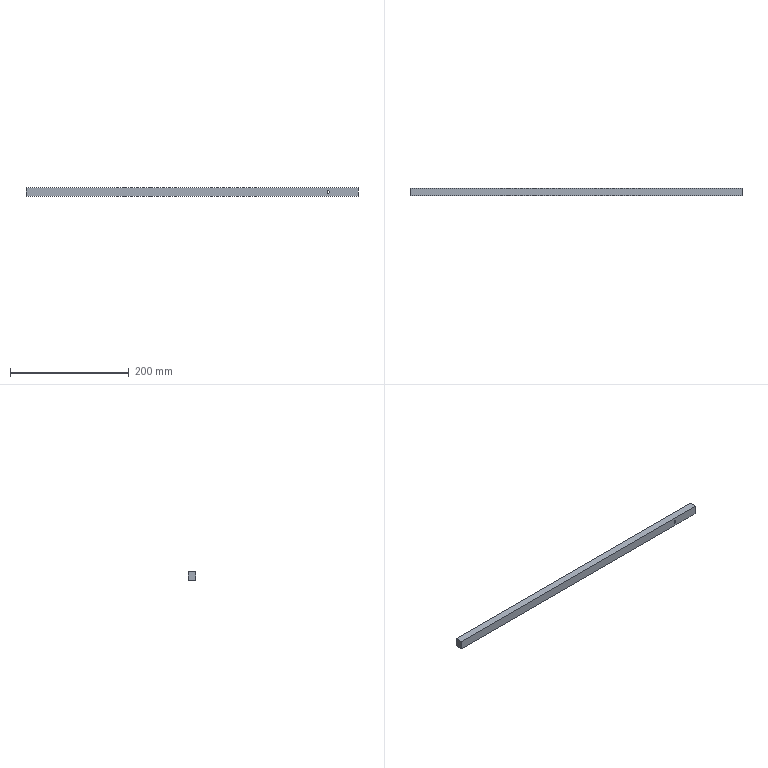Part | NX | 1 solid | 9 faces | box 560 x 12.5 x 15 mm | volume 104651 mm3 | plane 7 | cylinder 2 | commonest cylinder face diameters 4.5 x1 7.5 x1
STEP:
#1=CARTESIAN_POINT('',(510.,-6.25,-2.25));
#2=VERTEX_POINT('',#1);
#3=CARTESIAN_POINT('',(510.,-6.25,0.));
#4=DIRECTION('',(0.,-1.,0.));
#5=DIRECTION('',(0.,0.,-1.));
#6=AXIS2_PLACEMENT_3D('',#3,#4,#5);
#7=CIRCLE('',#6,2.25);
#8=EDGE_CURVE('',#2,#2,#7,.T.);
#9=ORIENTED_EDGE('',*,*,#8,.F.);
#10=EDGE_LOOP('',(#9));
#11=FACE_BOUND('',#10,.T.);
#12=CARTESIAN_POINT('',(560.,-6.25,7.5));
#13=VERTEX_POINT('',#12);
#14=CARTESIAN_POINT('',(560.,-6.25,-7.5));
#15=VERTEX_POINT('',#14);
#16=CARTESIAN_POINT('',(560.,-6.25,7.5));
#17=DIRECTION('',(0.,0.,-1.));
#18=VECTOR('',#17,1.);
#19=LINE('',#16,#18);
#20=EDGE_CURVE('',#13,#15,#19,.T.);
#21=ORIENTED_EDGE('',*,*,#20,.F.);
#22=CARTESIAN_POINT('',(0.,-6.25,7.5));
#23=VERTEX_POINT('',#22);
#24=CARTESIAN_POINT('',(0.,-6.25,7.5));
#25=DIRECTION('',(1.,0.,0.));
#26=VECTOR('',#25,1.);
#27=LINE('',#24,#26);
#28=EDGE_CURVE('',#23,#13,#27,.T.);
#29=ORIENTED_EDGE('',*,*,#28,.F.);
#30=CARTESIAN_POINT('',(0.,-6.25,-7.5));
#31=VERTEX_POINT('',#30);
#32=CARTESIAN_POINT('',(0.,-6.25,7.5));
#33=DIRECTION('',(0.,0.,-1.));
#34=VECTOR('',#33,1.);
#35=LINE('',#32,#34);
#36=EDGE_CURVE('',#23,#31,#35,.T.);
#37=ORIENTED_EDGE('',*,*,#36,.T.);
#38=CARTESIAN_POINT('',(0.,-6.25,-7.5));
#39=DIRECTION('',(1.,0.,0.));
#40=VECTOR('',#39,1.);
#41=LINE('',#38,#40);
#42=EDGE_CURVE('',#31,#15,#41,.T.);
#43=ORIENTED_EDGE('',*,*,#42,.T.);
#44=EDGE_LOOP('',(#21,#29,#37,#43));
#45=FACE_BOUND('',#44,.T.);
#46=CARTESIAN_POINT('',(0.,-6.25,7.5));
#47=DIRECTION('',(0.,-1.,0.));
#48=DIRECTION('',(0.,0.,1.));
#49=AXIS2_PLACEMENT_3D('',#46,#47,#48);
#50=PLANE('',#49);
#51=ADVANCED_FACE('',(#11,#45),#50,.T.);
#52=CARTESIAN_POINT('',(560.,6.25,-7.5));
#53=VERTEX_POINT('',#52);
#54=CARTESIAN_POINT('',(560.,-6.25,-7.5));
#55=DIRECTION('',(0.,1.,0.));
#56=VECTOR('',#55,1.);
#57=LINE('',#54,#56);
#58=EDGE_CURVE('',#15,#53,#57,.T.);
#59=ORIENTED_EDGE('',*,*,#58,.F.);
#60=ORIENTED_EDGE('',*,*,#42,.F.);
#61=CARTESIAN_POINT('',(0.,6.25,-7.5));
#62=VERTEX_POINT('',#61);
#63=CARTESIAN_POINT('',(0.,-6.25,-7.5));
#64=DIRECTION('',(0.,1.,0.));
#65=VECTOR('',#64,1.);
#66=LINE('',#63,#65);
#67=EDGE_CURVE('',#31,#62,#66,.T.);
#68=ORIENTED_EDGE('',*,*,#67,.T.);
#69=CARTESIAN_POINT('',(0.,6.25,-7.5));
#70=DIRECTION('',(1.,0.,0.));
#71=VECTOR('',#70,1.);
#72=LINE('',#69,#71);
#73=EDGE_CURVE('',#62,#53,#72,.T.);
#74=ORIENTED_EDGE('',*,*,#73,.T.);
#75=EDGE_LOOP('',(#59,#60,#68,#74));
#76=FACE_OUTER_BOUND('',#75,.T.);
#77=CARTESIAN_POINT('',(0.,-6.25,-7.5));
#78=DIRECTION('',(0.,0.,-1.));
#79=DIRECTION('',(1.,0.,0.));
#80=AXIS2_PLACEMENT_3D('',#77,#78,#79);
#81=PLANE('',#80);
#82=ADVANCED_FACE('',(#76),#81,.T.);
#83=CARTESIAN_POINT('',(510.,6.25,-3.75));
#84=VERTEX_POINT('',#83);
#85=CARTESIAN_POINT('',(510.,6.25,0.));
#86=DIRECTION('',(0.,-1.,0.));
#87=DIRECTION('',(0.,0.,-1.));
#88=AXIS2_PLACEMENT_3D('',#85,#86,#87);
#89=CIRCLE('',#88,3.75);
#90=EDGE_CURVE('',#84,#84,#89,.T.);
#91=ORIENTED_EDGE('',*,*,#90,.T.);
#92=EDGE_LOOP('',(#91));
#93=FACE_BOUND('',#92,.T.);
#94=CARTESIAN_POINT('',(560.,6.25,7.5));
#95=VERTEX_POINT('',#94);
#96=CARTESIAN_POINT('',(560.,6.25,-7.5));
#97=DIRECTION('',(0.,0.,1.));
#98=VECTOR('',#97,1.);
#99=LINE('',#96,#98);
#100=EDGE_CURVE('',#53,#95,#99,.T.);
#101=ORIENTED_EDGE('',*,*,#100,.F.);
#102=ORIENTED_EDGE('',*,*,#73,.F.);
#103=CARTESIAN_POINT('',(0.,6.25,7.5));
#104=VERTEX_POINT('',#103);
#105=CARTESIAN_POINT('',(0.,6.25,-7.5));
#106=DIRECTION('',(0.,0.,1.));
#107=VECTOR('',#106,1.);
#108=LINE('',#105,#107);
#109=EDGE_CURVE('',#62,#104,#108,.T.);
#110=ORIENTED_EDGE('',*,*,#109,.T.);
#111=CARTESIAN_POINT('',(0.,6.25,7.5));
#112=DIRECTION('',(1.,0.,0.));
#113=VECTOR('',#112,1.);
#114=LINE('',#111,#113);
#115=EDGE_CURVE('',#104,#95,#114,.T.);
#116=ORIENTED_EDGE('',*,*,#115,.T.);
#117=EDGE_LOOP('',(#101,#102,#110,#116));
#118=FACE_BOUND('',#117,.T.);
#119=CARTESIAN_POINT('',(0.,6.25,-7.5));
#120=DIRECTION('',(0.,1.,0.));
#121=DIRECTION('',(0.,0.,-1.));
#122=AXIS2_PLACEMENT_3D('',#119,#120,#121);
#123=PLANE('',#122);
#124=ADVANCED_FACE('',(#93,#118),#123,.T.);
#125=CARTESIAN_POINT('',(560.,6.25,7.5));
#126=DIRECTION('',(0.,-1.,0.));
#127=VECTOR('',#126,1.);
#128=LINE('',#125,#127);
#129=EDGE_CURVE('',#95,#13,#128,.T.);
#130=ORIENTED_EDGE('',*,*,#129,.F.);
#131=ORIENTED_EDGE('',*,*,#115,.F.);
#132=CARTESIAN_POINT('',(0.,6.25,7.5));
#133=DIRECTION('',(0.,-1.,0.));
#134=VECTOR('',#133,1.);
#135=LINE('',#132,#134);
#136=EDGE_CURVE('',#104,#23,#135,.T.);
#137=ORIENTED_EDGE('',*,*,#136,.T.);
#138=ORIENTED_EDGE('',*,*,#28,.T.);
#139=EDGE_LOOP('',(#130,#131,#137,#138));
#140=FACE_OUTER_BOUND('',#139,.T.);
#141=CARTESIAN_POINT('',(0.,6.25,7.5));
#142=DIRECTION('',(0.,0.,1.));
#143=DIRECTION('',(-1.,0.,0.));
#144=AXIS2_PLACEMENT_3D('',#141,#142,#143);
#145=PLANE('',#144);
#146=ADVANCED_FACE('',(#140),#145,.T.);
#147=ORIENTED_EDGE('',*,*,#36,.F.);
#148=ORIENTED_EDGE('',*,*,#136,.F.);
#149=ORIENTED_EDGE('',*,*,#109,.F.);
#150=ORIENTED_EDGE('',*,*,#67,.F.);
#151=EDGE_LOOP('',(#147,#148,#149,#150));
#152=FACE_OUTER_BOUND('',#151,.T.);
#153=CARTESIAN_POINT('',(0.,0.,0.));
#154=DIRECTION('',(1.,0.,0.));
#155=DIRECTION('',(0.,0.,1.));
#156=AXIS2_PLACEMENT_3D('',#153,#154,#155);
#157=PLANE('',#156);
#158=ADVANCED_FACE('',(#152),#157,.F.);
#159=ORIENTED_EDGE('',*,*,#20,.T.);
#160=ORIENTED_EDGE('',*,*,#58,.T.);
#161=ORIENTED_EDGE('',*,*,#100,.T.);
#162=ORIENTED_EDGE('',*,*,#129,.T.);
#163=EDGE_LOOP('',(#159,#160,#161,#162));
#164=FACE_OUTER_BOUND('',#163,.T.);
#165=CARTESIAN_POINT('',(560.,0.,0.));
#166=DIRECTION('',(1.,0.,0.));
#167=DIRECTION('',(0.,0.,1.));
#168=AXIS2_PLACEMENT_3D('',#165,#166,#167);
#169=PLANE('',#168);
#170=ADVANCED_FACE('',(#164),#169,.T.);
#171=CARTESIAN_POINT('',(510.,0.95,-2.25));
#172=VERTEX_POINT('',#171);
#173=CARTESIAN_POINT('',(510.,0.95,0.));
#174=DIRECTION('',(0.,1.,0.));
#175=DIRECTION('',(0.,0.,-1.));
#176=AXIS2_PLACEMENT_3D('',#173,#174,#175);
#177=CIRCLE('',#176,2.25);
#178=EDGE_CURVE('',#172,#172,#177,.T.);
#179=ORIENTED_EDGE('',*,*,#178,.T.);
#180=EDGE_LOOP('',(#179));
#181=FACE_BOUND('',#180,.T.);
#182=ORIENTED_EDGE('',*,*,#8,.T.);
#183=EDGE_LOOP('',(#182));
#184=FACE_BOUND('',#183,.T.);
#185=CARTESIAN_POINT('',(510.,6.25,0.));
#186=DIRECTION('',(0.,-1.,0.));
#187=DIRECTION('',(0.,0.,1.));
#188=AXIS2_PLACEMENT_3D('',#185,#186,#187);
#189=CYLINDRICAL_SURFACE('',#188,2.25);
#190=ADVANCED_FACE('',(#181,#184),#189,.F.);
#191=CARTESIAN_POINT('',(510.,0.95,-3.75));
#192=VERTEX_POINT('',#191);
#193=CARTESIAN_POINT('',(510.,0.95,0.));
#194=DIRECTION('',(0.,1.,0.));
#195=DIRECTION('',(0.,0.,-1.));
#196=AXIS2_PLACEMENT_3D('',#193,#194,#195);
#197=CIRCLE('',#196,3.75);
#198=EDGE_CURVE('',#192,#192,#197,.T.);
#199=ORIENTED_EDGE('',*,*,#198,.T.);
#200=EDGE_LOOP('',(#199));
#201=FACE_BOUND('',#200,.T.);
#202=ORIENTED_EDGE('',*,*,#178,.F.);
#203=EDGE_LOOP('',(#202));
#204=FACE_BOUND('',#203,.T.);
#205=CARTESIAN_POINT('',(510.,0.95,0.));
#206=DIRECTION('',(0.,-1.,0.));
#207=DIRECTION('',(0.,0.,1.));
#208=AXIS2_PLACEMENT_3D('',#205,#206,#207);
#209=PLANE('',#208);
#210=ADVANCED_FACE('',(#201,#204),#209,.F.);
#211=ORIENTED_EDGE('',*,*,#198,.F.);
#212=EDGE_LOOP('',(#211));
#213=FACE_BOUND('',#212,.T.);
#214=ORIENTED_EDGE('',*,*,#90,.F.);
#215=EDGE_LOOP('',(#214));
#216=FACE_BOUND('',#215,.T.);
#217=CARTESIAN_POINT('',(510.,6.25,0.));
#218=DIRECTION('',(0.,-1.,0.));
#219=DIRECTION('',(0.,0.,1.));
#220=AXIS2_PLACEMENT_3D('',#217,#218,#219);
#221=CYLINDRICAL_SURFACE('',#220,3.75);
#222=ADVANCED_FACE('',(#213,#216),#221,.F.);
#223=CLOSED_SHELL('',(#51,#82,#124,#146,#158,#170,#190,#210,#222));
#224=MANIFOLD_SOLID_BREP('',#223);
#225=(LENGTH_UNIT()NAMED_UNIT(*)SI_UNIT(.MILLI.,.METRE.));
#226=UNCERTAINTY_MEASURE_WITH_UNIT(LENGTH_MEASURE(0.00002),#225,'','');
#227=(NAMED_UNIT(*)PLANE_ANGLE_UNIT()SI_UNIT($,.RADIAN.));
#228=PLANE_ANGLE_MEASURE_WITH_UNIT(PLANE_ANGLE_MEASURE(0.01745),#227);
#229=DIMENSIONAL_EXPONENTS(0.,0.,0.,0.,0.,0.,0.);
#230=(CONVERSION_BASED_UNIT('DEGREE',#228)NAMED_UNIT(#229)PLANE_ANGLE_UNIT());
#231=(NAMED_UNIT(*)SI_UNIT($,.STERADIAN.)SOLID_ANGLE_UNIT());
#232=(GEOMETRIC_REPRESENTATION_CONTEXT(3)GLOBAL_UNCERTAINTY_ASSIGNED_CONTEXT((#226))GLOBAL_UNIT_ASSIGNED_CONTEXT((#225,#230,#231))REPRESENTATION_CONTEXT('',''));
#233=ADVANCED_BREP_SHAPE_REPRESENTATION('',(#224),#232);